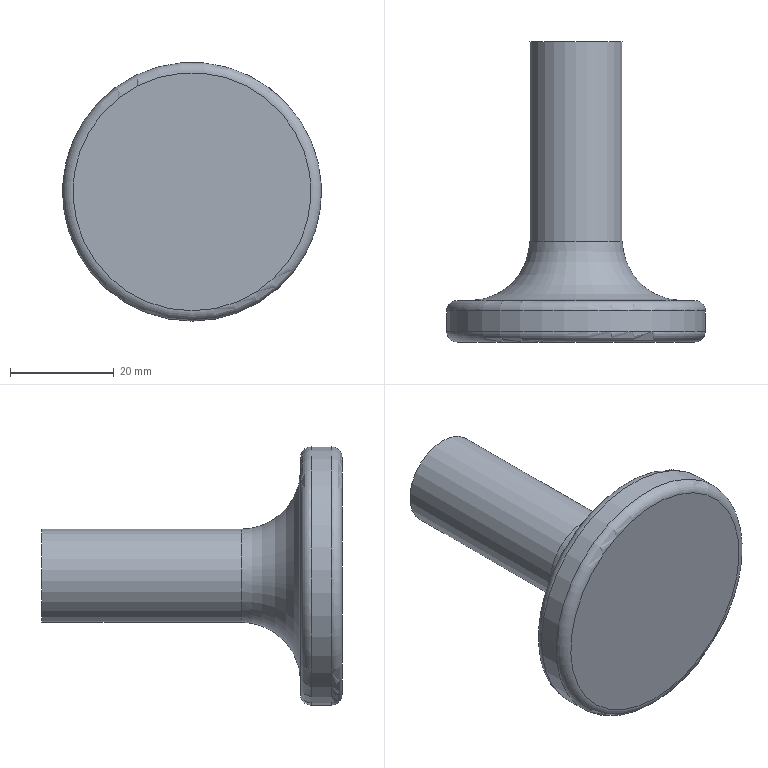Part | NX | 1 solid | 8 faces | box 50 x 58 x 50 mm | volume 30230 mm3 | plane 3 | torus 3 | cylinder 2 | commonest cylinder face diameters 18 x1 50 x1
STEP:
#1=CARTESIAN_POINT('',(5325.348,245.931,-317.999));
#2=VERTEX_POINT('',#1);
#3=CARTESIAN_POINT('',(5325.348,245.931,-308.999));
#4=DIRECTION('',(0.,1.,0.));
#5=DIRECTION('',(0.,0.,-1.));
#6=AXIS2_PLACEMENT_3D('',#3,#4,#5);
#7=CIRCLE('',#6,9.);
#8=EDGE_CURVE('',#2,#2,#7,.T.);
#9=ORIENTED_EDGE('',*,*,#8,.T.);
#10=EDGE_LOOP('',(#9));
#11=FACE_BOUND('',#10,.T.);
#12=CARTESIAN_POINT('',(5325.348,284.431,-299.999));
#13=VERTEX_POINT('',#12);
#14=CARTESIAN_POINT('',(5325.348,284.431,-308.999));
#15=DIRECTION('',(0.,1.,0.));
#16=DIRECTION('',(0.,0.,1.));
#17=AXIS2_PLACEMENT_3D('',#14,#15,#16);
#18=CIRCLE('',#17,9.);
#19=EDGE_CURVE('',#13,#13,#18,.T.);
#20=ORIENTED_EDGE('',*,*,#19,.F.);
#21=EDGE_LOOP('',(#20));
#22=FACE_BOUND('',#21,.T.);
#23=CARTESIAN_POINT('',(5325.348,234.431,-308.999));
#24=DIRECTION('',(0.,1.,0.));
#25=DIRECTION('',(0.,0.,1.));
#26=AXIS2_PLACEMENT_3D('',#23,#24,#25);
#27=CYLINDRICAL_SURFACE('',#26,9.);
#28=ADVANCED_FACE('',(#11,#22),#27,.T.);
#29=ORIENTED_EDGE('',*,*,#19,.T.);
#30=EDGE_LOOP('',(#29));
#31=FACE_OUTER_BOUND('',#30,.T.);
#32=CARTESIAN_POINT('',(5325.348,284.431,-308.999));
#33=DIRECTION('',(0.,1.,0.));
#34=DIRECTION('',(0.,0.,1.));
#35=AXIS2_PLACEMENT_3D('',#32,#33,#34);
#36=PLANE('',#35);
#37=ADVANCED_FACE('',(#31),#36,.T.);
#38=CARTESIAN_POINT('',(5325.348,228.431,-333.999));
#39=VERTEX_POINT('',#38);
#40=CARTESIAN_POINT('',(5325.348,228.431,-308.999));
#41=DIRECTION('',(0.,1.,0.));
#42=DIRECTION('',(0.,0.,-1.));
#43=AXIS2_PLACEMENT_3D('',#40,#41,#42);
#44=CIRCLE('',#43,25.);
#45=EDGE_CURVE('',#39,#39,#44,.T.);
#46=ORIENTED_EDGE('',*,*,#45,.T.);
#47=EDGE_LOOP('',(#46));
#48=FACE_BOUND('',#47,.T.);
#49=CARTESIAN_POINT('',(5325.348,232.431,-333.999));
#50=VERTEX_POINT('',#49);
#51=CARTESIAN_POINT('',(5325.348,232.431,-308.999));
#52=DIRECTION('',(0.,-1.,0.));
#53=DIRECTION('',(0.,0.,-1.));
#54=AXIS2_PLACEMENT_3D('',#51,#52,#53);
#55=CIRCLE('',#54,25.);
#56=EDGE_CURVE('',#50,#50,#55,.T.);
#57=ORIENTED_EDGE('',*,*,#56,.T.);
#58=EDGE_LOOP('',(#57));
#59=FACE_BOUND('',#58,.T.);
#60=CARTESIAN_POINT('',(5325.348,226.431,-308.999));
#61=DIRECTION('',(0.,1.,0.));
#62=DIRECTION('',(0.,0.,1.));
#63=AXIS2_PLACEMENT_3D('',#60,#61,#62);
#64=CYLINDRICAL_SURFACE('',#63,25.);
#65=ADVANCED_FACE('',(#48,#59),#64,.T.);
#66=CARTESIAN_POINT('',(5325.348,226.431,-331.999));
#67=VERTEX_POINT('',#66);
#68=CARTESIAN_POINT('',(5325.348,226.431,-308.999));
#69=DIRECTION('',(0.,-1.,0.));
#70=DIRECTION('',(0.,0.,-1.));
#71=AXIS2_PLACEMENT_3D('',#68,#69,#70);
#72=CIRCLE('',#71,23.);
#73=EDGE_CURVE('',#67,#67,#72,.T.);
#74=ORIENTED_EDGE('',*,*,#73,.T.);
#75=EDGE_LOOP('',(#74));
#76=FACE_OUTER_BOUND('',#75,.T.);
#77=CARTESIAN_POINT('',(5325.348,226.431,-308.999));
#78=DIRECTION('',(0.,-1.,0.));
#79=DIRECTION('',(0.,0.,-1.));
#80=AXIS2_PLACEMENT_3D('',#77,#78,#79);
#81=PLANE('',#80);
#82=ADVANCED_FACE('',(#76),#81,.T.);
#83=CARTESIAN_POINT('',(5325.348,234.431,-329.499));
#84=VERTEX_POINT('',#83);
#85=CARTESIAN_POINT('',(5325.348,234.431,-308.999));
#86=DIRECTION('',(0.,-1.,0.));
#87=DIRECTION('',(0.,0.,-1.));
#88=AXIS2_PLACEMENT_3D('',#85,#86,#87);
#89=CIRCLE('',#88,20.5);
#90=EDGE_CURVE('',#84,#84,#89,.T.);
#91=ORIENTED_EDGE('',*,*,#90,.T.);
#92=EDGE_LOOP('',(#91));
#93=FACE_BOUND('',#92,.T.);
#94=CARTESIAN_POINT('',(5325.348,234.431,-331.999));
#95=VERTEX_POINT('',#94);
#96=CARTESIAN_POINT('',(5325.348,234.431,-308.999));
#97=DIRECTION('',(0.,1.,0.));
#98=DIRECTION('',(0.,0.,-1.));
#99=AXIS2_PLACEMENT_3D('',#96,#97,#98);
#100=CIRCLE('',#99,23.);
#101=EDGE_CURVE('',#95,#95,#100,.T.);
#102=ORIENTED_EDGE('',*,*,#101,.T.);
#103=EDGE_LOOP('',(#102));
#104=FACE_BOUND('',#103,.T.);
#105=CARTESIAN_POINT('',(5325.348,234.431,-308.999));
#106=DIRECTION('',(0.,-1.,0.));
#107=DIRECTION('',(0.,0.,-1.));
#108=AXIS2_PLACEMENT_3D('',#105,#106,#107);
#109=PLANE('',#108);
#110=ADVANCED_FACE('',(#93,#104),#109,.F.);
#111=ORIENTED_EDGE('',*,*,#45,.F.);
#112=EDGE_LOOP('',(#111));
#113=FACE_BOUND('',#112,.T.);
#114=ORIENTED_EDGE('',*,*,#73,.F.);
#115=EDGE_LOOP('',(#114));
#116=FACE_BOUND('',#115,.T.);
#117=CARTESIAN_POINT('',(5325.348,228.431,-308.999));
#118=DIRECTION('',(0.,-1.,0.));
#119=DIRECTION('',(0.,0.,-1.));
#120=AXIS2_PLACEMENT_3D('',#117,#118,#119);
#121=TOROIDAL_SURFACE('',#120,23.,2.);
#122=ADVANCED_FACE('',(#113,#116),#121,.T.);
#123=ORIENTED_EDGE('',*,*,#101,.F.);
#124=EDGE_LOOP('',(#123));
#125=FACE_BOUND('',#124,.T.);
#126=ORIENTED_EDGE('',*,*,#56,.F.);
#127=EDGE_LOOP('',(#126));
#128=FACE_BOUND('',#127,.T.);
#129=CARTESIAN_POINT('',(5325.348,232.431,-308.999));
#130=DIRECTION('',(0.,-1.,0.));
#131=DIRECTION('',(0.,0.,-1.));
#132=AXIS2_PLACEMENT_3D('',#129,#130,#131);
#133=TOROIDAL_SURFACE('',#132,23.,2.);
#134=ADVANCED_FACE('',(#125,#128),#133,.T.);
#135=ORIENTED_EDGE('',*,*,#90,.F.);
#136=EDGE_LOOP('',(#135));
#137=FACE_BOUND('',#136,.T.);
#138=ORIENTED_EDGE('',*,*,#8,.F.);
#139=EDGE_LOOP('',(#138));
#140=FACE_BOUND('',#139,.T.);
#141=CARTESIAN_POINT('',(5325.348,245.931,-308.999));
#142=DIRECTION('',(0.,-1.,0.));
#143=DIRECTION('',(0.,0.,-1.));
#144=AXIS2_PLACEMENT_3D('',#141,#142,#143);
#145=TOROIDAL_SURFACE('',#144,20.5,11.5);
#146=ADVANCED_FACE('',(#137,#140),#145,.F.);
#147=CLOSED_SHELL('',(#28,#37,#65,#82,#110,#122,#134,#146));
#148=MANIFOLD_SOLID_BREP('',#147);
#149=(LENGTH_UNIT()NAMED_UNIT(*)SI_UNIT(.MILLI.,.METRE.));
#150=UNCERTAINTY_MEASURE_WITH_UNIT(LENGTH_MEASURE(0.00002),#149,'','');
#151=(NAMED_UNIT(*)PLANE_ANGLE_UNIT()SI_UNIT($,.RADIAN.));
#152=PLANE_ANGLE_MEASURE_WITH_UNIT(PLANE_ANGLE_MEASURE(0.01745),#151);
#153=DIMENSIONAL_EXPONENTS(0.,0.,0.,0.,0.,0.,0.);
#154=(CONVERSION_BASED_UNIT('DEGREE',#152)NAMED_UNIT(#153)PLANE_ANGLE_UNIT());
#155=(NAMED_UNIT(*)SI_UNIT($,.STERADIAN.)SOLID_ANGLE_UNIT());
#156=(GEOMETRIC_REPRESENTATION_CONTEXT(3)GLOBAL_UNCERTAINTY_ASSIGNED_CONTEXT((#150))GLOBAL_UNIT_ASSIGNED_CONTEXT((#149,#154,#155))REPRESENTATION_CONTEXT('',''));
#157=ADVANCED_BREP_SHAPE_REPRESENTATION('',(#148),#156);